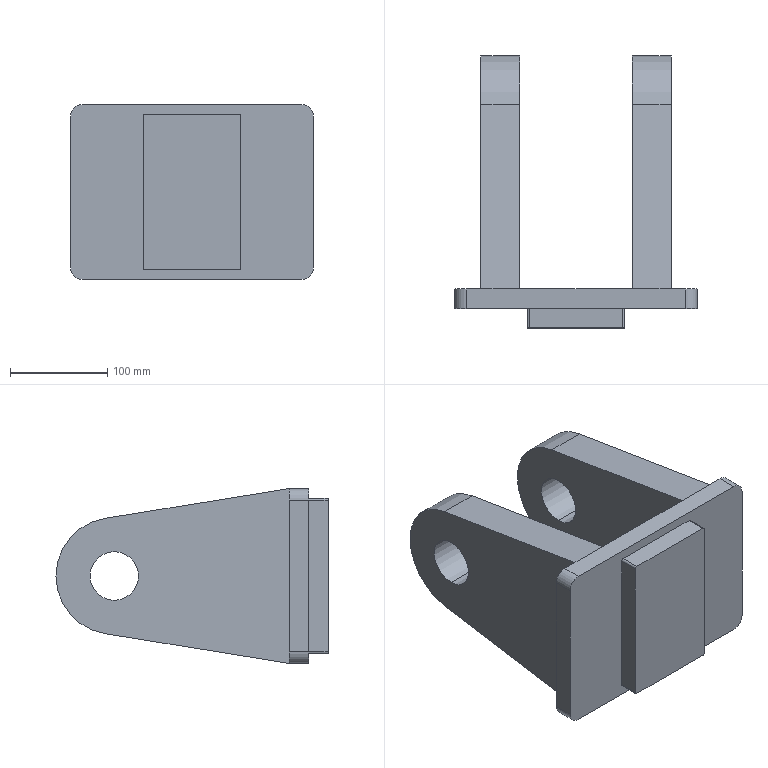Part | SolidWorks | features ICE 2, Extrusion 1, MirrorPattern 1 | 1 solid | 35 faces | box 250 x 280 x 180 mm | volume 3684479 mm3 | plane 21 | cylinder 14 | commonest cylinder face diameters 4 x4 24 x4 50 x4 120 x2
STEP:
#1=CARTESIAN_POINT('',(-98.,200.,25.));
#2=VERTEX_POINT('',#1);
#3=CARTESIAN_POINT('',(-98.,200.,-25.));
#4=VERTEX_POINT('',#3);
#5=CARTESIAN_POINT('',(-98.,200.,0.));
#6=DIRECTION('',(1.,0.,0.));
#7=DIRECTION('',(0.,0.,-1.));
#8=AXIS2_PLACEMENT_3D('',#5,#6,#7);
#9=CIRCLE('',#8,25.);
#10=EDGE_CURVE('',#2,#4,#9,.T.);
#11=ORIENTED_EDGE('',*,*,#10,.F.);
#12=CARTESIAN_POINT('',(-58.,200.,25.));
#13=VERTEX_POINT('',#12);
#14=CARTESIAN_POINT('',(-98.,200.,25.));
#15=DIRECTION('',(1.,0.,0.));
#16=VECTOR('',#15,1000.);
#17=LINE('',#14,#16);
#18=EDGE_CURVE('',#2,#13,#17,.T.);
#19=ORIENTED_EDGE('',*,*,#18,.T.);
#20=CARTESIAN_POINT('',(-58.,200.,-25.));
#21=VERTEX_POINT('',#20);
#22=CARTESIAN_POINT('',(-58.,200.,0.));
#23=DIRECTION('',(1.,0.,0.));
#24=DIRECTION('',(0.,0.,-1.));
#25=AXIS2_PLACEMENT_3D('',#22,#23,#24);
#26=CIRCLE('',#25,25.);
#27=EDGE_CURVE('',#13,#21,#26,.T.);
#28=ORIENTED_EDGE('',*,*,#27,.T.);
#29=CARTESIAN_POINT('',(-98.,200.,-25.));
#30=DIRECTION('',(1.,0.,0.));
#31=VECTOR('',#30,1000.);
#32=LINE('',#29,#31);
#33=EDGE_CURVE('',#4,#21,#32,.T.);
#34=ORIENTED_EDGE('',*,*,#33,.F.);
#35=EDGE_LOOP('',(#11,#19,#28,#34));
#36=FACE_OUTER_BOUND('',#35,.T.);
#37=CARTESIAN_POINT('',(-98.,200.,0.));
#38=DIRECTION('',(1.,0.,0.));
#39=DIRECTION('',(0.,0.,-1.));
#40=AXIS2_PLACEMENT_3D('',#37,#38,#39);
#41=CYLINDRICAL_SURFACE('',#40,25.);
#42=ADVANCED_FACE('',(#36),#41,.F.);
#43=CARTESIAN_POINT('',(98.,200.,25.));
#44=VERTEX_POINT('',#43);
#45=CARTESIAN_POINT('',(98.,200.,-25.));
#46=VERTEX_POINT('',#45);
#47=CARTESIAN_POINT('',(98.,200.,0.));
#48=DIRECTION('',(1.,0.,0.));
#49=DIRECTION('',(0.,0.,-1.));
#50=AXIS2_PLACEMENT_3D('',#47,#48,#49);
#51=CIRCLE('',#50,25.);
#52=EDGE_CURVE('',#44,#46,#51,.T.);
#53=ORIENTED_EDGE('',*,*,#52,.T.);
#54=CARTESIAN_POINT('',(58.,200.,-25.));
#55=VERTEX_POINT('',#54);
#56=CARTESIAN_POINT('',(98.,200.,-25.));
#57=DIRECTION('',(-1.,0.,0.));
#58=VECTOR('',#57,1000.);
#59=LINE('',#56,#58);
#60=EDGE_CURVE('',#46,#55,#59,.T.);
#61=ORIENTED_EDGE('',*,*,#60,.T.);
#62=CARTESIAN_POINT('',(58.,200.,25.));
#63=VERTEX_POINT('',#62);
#64=CARTESIAN_POINT('',(58.,200.,0.));
#65=DIRECTION('',(1.,0.,0.));
#66=DIRECTION('',(0.,0.,-1.));
#67=AXIS2_PLACEMENT_3D('',#64,#65,#66);
#68=CIRCLE('',#67,25.);
#69=EDGE_CURVE('',#63,#55,#68,.T.);
#70=ORIENTED_EDGE('',*,*,#69,.F.);
#71=CARTESIAN_POINT('',(98.,200.,25.));
#72=DIRECTION('',(-1.,0.,0.));
#73=VECTOR('',#72,1000.);
#74=LINE('',#71,#73);
#75=EDGE_CURVE('',#44,#63,#74,.T.);
#76=ORIENTED_EDGE('',*,*,#75,.F.);
#77=EDGE_LOOP('',(#53,#61,#70,#76));
#78=FACE_OUTER_BOUND('',#77,.T.);
#79=CARTESIAN_POINT('',(98.,200.,0.));
#80=DIRECTION('',(-1.,0.,0.));
#81=DIRECTION('',(0.,0.,1.));
#82=AXIS2_PLACEMENT_3D('',#79,#80,#81);
#83=CYLINDRICAL_SURFACE('',#82,25.);
#84=ADVANCED_FACE('',(#78),#83,.F.);
#85=CARTESIAN_POINT('',(58.,20.,-90.));
#86=VERTEX_POINT('',#85);
#87=CARTESIAN_POINT('',(-58.,20.,-90.));
#88=VERTEX_POINT('',#87);
#89=CARTESIAN_POINT('',(113.,20.,-90.));
#90=DIRECTION('',(-1.,0.,0.));
#91=VECTOR('',#90,1000.);
#92=LINE('',#89,#91);
#93=EDGE_CURVE('',#86,#88,#92,.T.);
#94=ORIENTED_EDGE('',*,*,#93,.T.);
#95=CARTESIAN_POINT('',(-58.,20.,90.));
#96=VERTEX_POINT('',#95);
#97=CARTESIAN_POINT('',(-58.,20.,90.));
#98=DIRECTION('',(0.,0.,-1.));
#99=VECTOR('',#98,1000.);
#100=LINE('',#97,#99);
#101=EDGE_CURVE('',#96,#88,#100,.T.);
#102=ORIENTED_EDGE('',*,*,#101,.F.);
#103=CARTESIAN_POINT('',(58.,20.,90.));
#104=VERTEX_POINT('',#103);
#105=CARTESIAN_POINT('',(113.,20.,90.));
#106=DIRECTION('',(1.,0.,0.));
#107=VECTOR('',#106,1000.);
#108=LINE('',#105,#107);
#109=EDGE_CURVE('',#96,#104,#108,.T.);
#110=ORIENTED_EDGE('',*,*,#109,.T.);
#111=CARTESIAN_POINT('',(58.,20.,90.));
#112=DIRECTION('',(0.,0.,-1.));
#113=VECTOR('',#112,1000.);
#114=LINE('',#111,#113);
#115=EDGE_CURVE('',#104,#86,#114,.T.);
#116=ORIENTED_EDGE('',*,*,#115,.T.);
#117=EDGE_LOOP('',(#94,#102,#110,#116));
#118=FACE_OUTER_BOUND('',#117,.T.);
#119=CARTESIAN_POINT('',(-113.,20.,-78.));
#120=DIRECTION('',(0.,1.,0.));
#121=DIRECTION('',(0.,0.,1.));
#122=AXIS2_PLACEMENT_3D('',#119,#120,#121);
#123=PLANE('',#122);
#124=ADVANCED_FACE('',(#118),#123,.T.);
#125=CARTESIAN_POINT('',(-98.,20.,90.));
#126=VERTEX_POINT('',#125);
#127=CARTESIAN_POINT('',(-98.,20.,-90.));
#128=VERTEX_POINT('',#127);
#129=CARTESIAN_POINT('',(-98.,20.,90.));
#130=DIRECTION('',(0.,0.,-1.));
#131=VECTOR('',#130,1000.);
#132=LINE('',#129,#131);
#133=EDGE_CURVE('',#126,#128,#132,.T.);
#134=ORIENTED_EDGE('',*,*,#133,.T.);
#135=CARTESIAN_POINT('',(-113.,20.,-90.));
#136=VERTEX_POINT('',#135);
#137=CARTESIAN_POINT('',(113.,20.,-90.));
#138=DIRECTION('',(-1.,0.,0.));
#139=VECTOR('',#138,1000.);
#140=LINE('',#137,#139);
#141=EDGE_CURVE('',#128,#136,#140,.T.);
#142=ORIENTED_EDGE('',*,*,#141,.T.);
#143=CARTESIAN_POINT('',(-125.,20.,-78.));
#144=VERTEX_POINT('',#143);
#145=CARTESIAN_POINT('',(-113.,20.,-78.));
#146=DIRECTION('',(0.,1.,0.));
#147=DIRECTION('',(0.,0.,1.));
#148=AXIS2_PLACEMENT_3D('',#145,#146,#147);
#149=CIRCLE('',#148,12.);
#150=EDGE_CURVE('',#136,#144,#149,.T.);
#151=ORIENTED_EDGE('',*,*,#150,.T.);
#152=CARTESIAN_POINT('',(-125.,20.,78.));
#153=VERTEX_POINT('',#152);
#154=CARTESIAN_POINT('',(-125.,20.,-78.));
#155=DIRECTION('',(0.,0.,1.));
#156=VECTOR('',#155,1000.);
#157=LINE('',#154,#156);
#158=EDGE_CURVE('',#144,#153,#157,.T.);
#159=ORIENTED_EDGE('',*,*,#158,.T.);
#160=CARTESIAN_POINT('',(-113.,20.,90.));
#161=VERTEX_POINT('',#160);
#162=CARTESIAN_POINT('',(-113.,20.,78.));
#163=DIRECTION('',(0.,1.,0.));
#164=DIRECTION('',(0.,0.,-1.));
#165=AXIS2_PLACEMENT_3D('',#162,#163,#164);
#166=CIRCLE('',#165,12.);
#167=EDGE_CURVE('',#153,#161,#166,.T.);
#168=ORIENTED_EDGE('',*,*,#167,.T.);
#169=CARTESIAN_POINT('',(113.,20.,90.));
#170=DIRECTION('',(1.,0.,0.));
#171=VECTOR('',#170,1000.);
#172=LINE('',#169,#171);
#173=EDGE_CURVE('',#161,#126,#172,.T.);
#174=ORIENTED_EDGE('',*,*,#173,.T.);
#175=EDGE_LOOP('',(#134,#142,#151,#159,#168,#174));
#176=FACE_OUTER_BOUND('',#175,.T.);
#177=CARTESIAN_POINT('',(-113.,20.,-78.));
#178=DIRECTION('',(0.,1.,0.));
#179=DIRECTION('',(0.,0.,1.));
#180=AXIS2_PLACEMENT_3D('',#177,#178,#179);
#181=PLANE('',#180);
#182=ADVANCED_FACE('',(#176),#181,.T.);
#183=CARTESIAN_POINT('',(-113.,0.,-90.));
#184=VERTEX_POINT('',#183);
#185=CARTESIAN_POINT('',(-125.,0.,-78.));
#186=VERTEX_POINT('',#185);
#187=CARTESIAN_POINT('',(-113.,0.,-78.));
#188=DIRECTION('',(0.,1.,0.));
#189=DIRECTION('',(0.,0.,1.));
#190=AXIS2_PLACEMENT_3D('',#187,#188,#189);
#191=CIRCLE('',#190,12.);
#192=EDGE_CURVE('',#184,#186,#191,.T.);
#193=ORIENTED_EDGE('',*,*,#192,.F.);
#194=CARTESIAN_POINT('',(113.,0.,-90.));
#195=VERTEX_POINT('',#194);
#196=CARTESIAN_POINT('',(113.,0.,-90.));
#197=DIRECTION('',(-1.,0.,0.));
#198=VECTOR('',#197,1000.);
#199=LINE('',#196,#198);
#200=EDGE_CURVE('',#195,#184,#199,.T.);
#201=ORIENTED_EDGE('',*,*,#200,.F.);
#202=CARTESIAN_POINT('',(125.,0.,-78.));
#203=VERTEX_POINT('',#202);
#204=CARTESIAN_POINT('',(113.,0.,-78.));
#205=DIRECTION('',(0.,1.,0.));
#206=DIRECTION('',(0.,0.,-1.));
#207=AXIS2_PLACEMENT_3D('',#204,#205,#206);
#208=CIRCLE('',#207,12.);
#209=EDGE_CURVE('',#203,#195,#208,.T.);
#210=ORIENTED_EDGE('',*,*,#209,.F.);
#211=CARTESIAN_POINT('',(125.,0.,78.));
#212=VERTEX_POINT('',#211);
#213=CARTESIAN_POINT('',(125.,0.,-78.));
#214=DIRECTION('',(0.,0.,-1.));
#215=VECTOR('',#214,1000.);
#216=LINE('',#213,#215);
#217=EDGE_CURVE('',#212,#203,#216,.T.);
#218=ORIENTED_EDGE('',*,*,#217,.F.);
#219=CARTESIAN_POINT('',(113.,0.,90.));
#220=VERTEX_POINT('',#219);
#221=CARTESIAN_POINT('',(113.,0.,78.));
#222=DIRECTION('',(0.,1.,0.));
#223=DIRECTION('',(0.,0.,1.));
#224=AXIS2_PLACEMENT_3D('',#221,#222,#223);
#225=CIRCLE('',#224,12.);
#226=EDGE_CURVE('',#220,#212,#225,.T.);
#227=ORIENTED_EDGE('',*,*,#226,.F.);
#228=CARTESIAN_POINT('',(-113.,0.,90.));
#229=VERTEX_POINT('',#228);
#230=CARTESIAN_POINT('',(113.,0.,90.));
#231=DIRECTION('',(1.,0.,0.));
#232=VECTOR('',#231,1000.);
#233=LINE('',#230,#232);
#234=EDGE_CURVE('',#229,#220,#233,.T.);
#235=ORIENTED_EDGE('',*,*,#234,.F.);
#236=CARTESIAN_POINT('',(-125.,0.,78.));
#237=VERTEX_POINT('',#236);
#238=CARTESIAN_POINT('',(-113.,0.,78.));
#239=DIRECTION('',(0.,1.,0.));
#240=DIRECTION('',(0.,0.,-1.));
#241=AXIS2_PLACEMENT_3D('',#238,#239,#240);
#242=CIRCLE('',#241,12.);
#243=EDGE_CURVE('',#237,#229,#242,.T.);
#244=ORIENTED_EDGE('',*,*,#243,.F.);
#245=CARTESIAN_POINT('',(-125.,0.,-78.));
#246=DIRECTION('',(0.,0.,1.));
#247=VECTOR('',#246,1000.);
#248=LINE('',#245,#247);
#249=EDGE_CURVE('',#186,#237,#248,.T.);
#250=ORIENTED_EDGE('',*,*,#249,.F.);
#251=EDGE_LOOP('',(#193,#201,#210,#218,#227,#235,#244,#250));
#252=FACE_OUTER_BOUND('',#251,.T.);
#253=CARTESIAN_POINT('',(-48.,0.,80.));
#254=VERTEX_POINT('',#253);
#255=CARTESIAN_POINT('',(-50.,0.,78.));
#256=VERTEX_POINT('',#255);
#257=CARTESIAN_POINT('',(-48.,0.,78.));
#258=DIRECTION('',(0.,-1.,0.));
#259=DIRECTION('',(0.,0.,-1.));
#260=AXIS2_PLACEMENT_3D('',#257,#258,#259);
#261=CIRCLE('',#260,2.);
#262=EDGE_CURVE('',#254,#256,#261,.T.);
#263=ORIENTED_EDGE('',*,*,#262,.F.);
#264=CARTESIAN_POINT('',(48.,0.,80.));
#265=VERTEX_POINT('',#264);
#266=CARTESIAN_POINT('',(48.,0.,80.));
#267=DIRECTION('',(-1.,0.,0.));
#268=VECTOR('',#267,1000.);
#269=LINE('',#266,#268);
#270=EDGE_CURVE('',#265,#254,#269,.T.);
#271=ORIENTED_EDGE('',*,*,#270,.F.);
#272=CARTESIAN_POINT('',(50.,0.,78.));
#273=VERTEX_POINT('',#272);
#274=CARTESIAN_POINT('',(48.,0.,78.));
#275=DIRECTION('',(0.,-1.,0.));
#276=DIRECTION('',(0.,0.,1.));
#277=AXIS2_PLACEMENT_3D('',#274,#275,#276);
#278=CIRCLE('',#277,2.);
#279=EDGE_CURVE('',#273,#265,#278,.T.);
#280=ORIENTED_EDGE('',*,*,#279,.F.);
#281=CARTESIAN_POINT('',(50.,0.,-78.));
#282=VERTEX_POINT('',#281);
#283=CARTESIAN_POINT('',(50.,0.,78.));
#284=DIRECTION('',(0.,0.,1.));
#285=VECTOR('',#284,1000.);
#286=LINE('',#283,#285);
#287=EDGE_CURVE('',#282,#273,#286,.T.);
#288=ORIENTED_EDGE('',*,*,#287,.F.);
#289=CARTESIAN_POINT('',(48.,0.,-80.));
#290=VERTEX_POINT('',#289);
#291=CARTESIAN_POINT('',(48.,0.,-78.));
#292=DIRECTION('',(0.,-1.,0.));
#293=DIRECTION('',(0.,0.,-1.));
#294=AXIS2_PLACEMENT_3D('',#291,#292,#293);
#295=CIRCLE('',#294,2.);
#296=EDGE_CURVE('',#290,#282,#295,.T.);
#297=ORIENTED_EDGE('',*,*,#296,.F.);
#298=CARTESIAN_POINT('',(-48.,0.,-80.));
#299=VERTEX_POINT('',#298);
#300=CARTESIAN_POINT('',(48.,0.,-80.));
#301=DIRECTION('',(1.,0.,0.));
#302=VECTOR('',#301,1000.);
#303=LINE('',#300,#302);
#304=EDGE_CURVE('',#299,#290,#303,.T.);
#305=ORIENTED_EDGE('',*,*,#304,.F.);
#306=CARTESIAN_POINT('',(-50.,0.,-78.));
#307=VERTEX_POINT('',#306);
#308=CARTESIAN_POINT('',(-48.,0.,-78.));
#309=DIRECTION('',(0.,-1.,0.));
#310=DIRECTION('',(0.,0.,1.));
#311=AXIS2_PLACEMENT_3D('',#308,#309,#310);
#312=CIRCLE('',#311,2.);
#313=EDGE_CURVE('',#307,#299,#312,.T.);
#314=ORIENTED_EDGE('',*,*,#313,.F.);
#315=CARTESIAN_POINT('',(-50.,0.,78.));
#316=DIRECTION('',(0.,0.,-1.));
#317=VECTOR('',#316,1000.);
#318=LINE('',#315,#317);
#319=EDGE_CURVE('',#256,#307,#318,.T.);
#320=ORIENTED_EDGE('',*,*,#319,.F.);
#321=EDGE_LOOP('',(#263,#271,#280,#288,#297,#305,#314,#320));
#322=FACE_BOUND('',#321,.T.);
#323=CARTESIAN_POINT('',(-113.,0.,-78.));
#324=DIRECTION('',(0.,1.,0.));
#325=DIRECTION('',(0.,0.,1.));
#326=AXIS2_PLACEMENT_3D('',#323,#324,#325);
#327=PLANE('',#326);
#328=ADVANCED_FACE('',(#252,#322),#327,.F.);
#329=ORIENTED_EDGE('',*,*,#192,.T.);
#330=CARTESIAN_POINT('',(-125.,20.,-78.));
#331=DIRECTION('',(0.,-1.,0.));
#332=VECTOR('',#331,1000.);
#333=LINE('',#330,#332);
#334=EDGE_CURVE('',#144,#186,#333,.T.);
#335=ORIENTED_EDGE('',*,*,#334,.F.);
#336=ORIENTED_EDGE('',*,*,#150,.F.);
#337=CARTESIAN_POINT('',(-113.,20.,-90.));
#338=DIRECTION('',(0.,-1.,0.));
#339=VECTOR('',#338,1000.);
#340=LINE('',#337,#339);
#341=EDGE_CURVE('',#136,#184,#340,.T.);
#342=ORIENTED_EDGE('',*,*,#341,.T.);
#343=EDGE_LOOP('',(#329,#335,#336,#342));
#344=FACE_OUTER_BOUND('',#343,.T.);
#345=CARTESIAN_POINT('',(-113.,20.,-78.));
#346=DIRECTION('',(0.,-1.,0.));
#347=DIRECTION('',(0.,0.,-1.));
#348=AXIS2_PLACEMENT_3D('',#345,#346,#347);
#349=CYLINDRICAL_SURFACE('',#348,12.);
#350=ADVANCED_FACE('',(#344),#349,.T.);
#351=ORIENTED_EDGE('',*,*,#249,.T.);
#352=CARTESIAN_POINT('',(-125.,20.,78.));
#353=DIRECTION('',(0.,-1.,0.));
#354=VECTOR('',#353,1000.);
#355=LINE('',#352,#354);
#356=EDGE_CURVE('',#153,#237,#355,.T.);
#357=ORIENTED_EDGE('',*,*,#356,.F.);
#358=ORIENTED_EDGE('',*,*,#158,.F.);
#359=ORIENTED_EDGE('',*,*,#334,.T.);
#360=EDGE_LOOP('',(#351,#357,#358,#359));
#361=FACE_OUTER_BOUND('',#360,.T.);
#362=CARTESIAN_POINT('',(-125.,20.,-78.));
#363=DIRECTION('',(1.,0.,0.));
#364=DIRECTION('',(0.,0.,-1.));
#365=AXIS2_PLACEMENT_3D('',#362,#363,#364);
#366=PLANE('',#365);
#367=ADVANCED_FACE('',(#361),#366,.F.);
#368=ORIENTED_EDGE('',*,*,#243,.T.);
#369=CARTESIAN_POINT('',(-113.,20.,90.));
#370=DIRECTION('',(0.,-1.,0.));
#371=VECTOR('',#370,1000.);
#372=LINE('',#369,#371);
#373=EDGE_CURVE('',#161,#229,#372,.T.);
#374=ORIENTED_EDGE('',*,*,#373,.F.);
#375=ORIENTED_EDGE('',*,*,#167,.F.);
#376=ORIENTED_EDGE('',*,*,#356,.T.);
#377=EDGE_LOOP('',(#368,#374,#375,#376));
#378=FACE_OUTER_BOUND('',#377,.T.);
#379=CARTESIAN_POINT('',(-113.,20.,78.));
#380=DIRECTION('',(0.,-1.,0.));
#381=DIRECTION('',(0.,0.,-1.));
#382=AXIS2_PLACEMENT_3D('',#379,#380,#381);
#383=CYLINDRICAL_SURFACE('',#382,12.);
#384=ADVANCED_FACE('',(#378),#383,.T.);
#385=ORIENTED_EDGE('',*,*,#234,.T.);
#386=CARTESIAN_POINT('',(113.,20.,90.));
#387=VERTEX_POINT('',#386);
#388=CARTESIAN_POINT('',(113.,20.,90.));
#389=DIRECTION('',(0.,-1.,0.));
#390=VECTOR('',#389,1000.);
#391=LINE('',#388,#390);
#392=EDGE_CURVE('',#387,#220,#391,.T.);
#393=ORIENTED_EDGE('',*,*,#392,.F.);
#394=CARTESIAN_POINT('',(98.,20.,90.));
#395=VERTEX_POINT('',#394);
#396=CARTESIAN_POINT('',(113.,20.,90.));
#397=DIRECTION('',(1.,0.,0.));
#398=VECTOR('',#397,1000.);
#399=LINE('',#396,#398);
#400=EDGE_CURVE('',#395,#387,#399,.T.);
#401=ORIENTED_EDGE('',*,*,#400,.F.);
#402=CARTESIAN_POINT('',(98.,20.,90.));
#403=DIRECTION('',(-1.,0.,0.));
#404=VECTOR('',#403,1000.);
#405=LINE('',#402,#404);
#406=EDGE_CURVE('',#395,#104,#405,.T.);
#407=ORIENTED_EDGE('',*,*,#406,.T.);
#408=ORIENTED_EDGE('',*,*,#109,.F.);
#409=CARTESIAN_POINT('',(-98.,20.,90.));
#410=DIRECTION('',(1.,0.,0.));
#411=VECTOR('',#410,1000.);
#412=LINE('',#409,#411);
#413=EDGE_CURVE('',#126,#96,#412,.T.);
#414=ORIENTED_EDGE('',*,*,#413,.F.);
#415=ORIENTED_EDGE('',*,*,#173,.F.);
#416=ORIENTED_EDGE('',*,*,#373,.T.);
#417=EDGE_LOOP('',(#385,#393,#401,#407,#408,#414,#415,#416));
#418=FACE_OUTER_BOUND('',#417,.T.);
#419=CARTESIAN_POINT('',(113.,20.,90.));
#420=DIRECTION('',(0.,0.,-1.));
#421=DIRECTION('',(-1.,0.,0.));
#422=AXIS2_PLACEMENT_3D('',#419,#420,#421);
#423=PLANE('',#422);
#424=ADVANCED_FACE('',(#418),#423,.F.);
#425=ORIENTED_EDGE('',*,*,#226,.T.);
#426=CARTESIAN_POINT('',(125.,20.,78.));
#427=VERTEX_POINT('',#426);
#428=CARTESIAN_POINT('',(125.,20.,78.));
#429=DIRECTION('',(0.,-1.,0.));
#430=VECTOR('',#429,1000.);
#431=LINE('',#428,#430);
#432=EDGE_CURVE('',#427,#212,#431,.T.);
#433=ORIENTED_EDGE('',*,*,#432,.F.);
#434=CARTESIAN_POINT('',(113.,20.,78.));
#435=DIRECTION('',(0.,1.,0.));
#436=DIRECTION('',(0.,0.,1.));
#437=AXIS2_PLACEMENT_3D('',#434,#435,#436);
#438=CIRCLE('',#437,12.);
#439=EDGE_CURVE('',#387,#427,#438,.T.);
#440=ORIENTED_EDGE('',*,*,#439,.F.);
#441=ORIENTED_EDGE('',*,*,#392,.T.);
#442=EDGE_LOOP('',(#425,#433,#440,#441));
#443=FACE_OUTER_BOUND('',#442,.T.);
#444=CARTESIAN_POINT('',(113.,20.,78.));
#445=DIRECTION('',(0.,-1.,0.));
#446=DIRECTION('',(0.,0.,-1.));
#447=AXIS2_PLACEMENT_3D('',#444,#445,#446);
#448=CYLINDRICAL_SURFACE('',#447,12.);
#449=ADVANCED_FACE('',(#443),#448,.T.);
#450=ORIENTED_EDGE('',*,*,#217,.T.);
#451=CARTESIAN_POINT('',(125.,20.,-78.));
#452=VERTEX_POINT('',#451);
#453=CARTESIAN_POINT('',(125.,20.,-78.));
#454=DIRECTION('',(0.,-1.,0.));
#455=VECTOR('',#454,1000.);
#456=LINE('',#453,#455);
#457=EDGE_CURVE('',#452,#203,#456,.T.);
#458=ORIENTED_EDGE('',*,*,#457,.F.);
#459=CARTESIAN_POINT('',(125.,20.,-78.));
#460=DIRECTION('',(0.,0.,-1.));
#461=VECTOR('',#460,1000.);
#462=LINE('',#459,#461);
#463=EDGE_CURVE('',#427,#452,#462,.T.);
#464=ORIENTED_EDGE('',*,*,#463,.F.);
#465=ORIENTED_EDGE('',*,*,#432,.T.);
#466=EDGE_LOOP('',(#450,#458,#464,#465));
#467=FACE_OUTER_BOUND('',#466,.T.);
#468=CARTESIAN_POINT('',(125.,20.,-78.));
#469=DIRECTION('',(-1.,0.,0.));
#470=DIRECTION('',(0.,0.,1.));
#471=AXIS2_PLACEMENT_3D('',#468,#469,#470);
#472=PLANE('',#471);
#473=ADVANCED_FACE('',(#467),#472,.F.);
#474=ORIENTED_EDGE('',*,*,#209,.T.);
#475=CARTESIAN_POINT('',(113.,20.,-90.));
#476=VERTEX_POINT('',#475);
#477=CARTESIAN_POINT('',(113.,20.,-90.));
#478=DIRECTION('',(0.,-1.,0.));
#479=VECTOR('',#478,1000.);
#480=LINE('',#477,#479);
#481=EDGE_CURVE('',#476,#195,#480,.T.);
#482=ORIENTED_EDGE('',*,*,#481,.F.);
#483=CARTESIAN_POINT('',(113.,20.,-78.));
#484=DIRECTION('',(0.,1.,0.));
#485=DIRECTION('',(0.,0.,-1.));
#486=AXIS2_PLACEMENT_3D('',#483,#484,#485);
#487=CIRCLE('',#486,12.);
#488=EDGE_CURVE('',#452,#476,#487,.T.);
#489=ORIENTED_EDGE('',*,*,#488,.F.);
#490=ORIENTED_EDGE('',*,*,#457,.T.);
#491=EDGE_LOOP('',(#474,#482,#489,#490));
#492=FACE_OUTER_BOUND('',#491,.T.);
#493=CARTESIAN_POINT('',(113.,20.,-78.));
#494=DIRECTION('',(0.,-1.,0.));
#495=DIRECTION('',(0.,0.,-1.));
#496=AXIS2_PLACEMENT_3D('',#493,#494,#495);
#497=CYLINDRICAL_SURFACE('',#496,12.);
#498=ADVANCED_FACE('',(#492),#497,.T.);
#499=ORIENTED_EDGE('',*,*,#200,.T.);
#500=ORIENTED_EDGE('',*,*,#341,.F.);
#501=ORIENTED_EDGE('',*,*,#141,.F.);
#502=CARTESIAN_POINT('',(-98.,20.,-90.));
#503=DIRECTION('',(1.,0.,0.));
#504=VECTOR('',#503,1000.);
#505=LINE('',#502,#504);
#506=EDGE_CURVE('',#128,#88,#505,.T.);
#507=ORIENTED_EDGE('',*,*,#506,.T.);
#508=ORIENTED_EDGE('',*,*,#93,.F.);
#509=CARTESIAN_POINT('',(98.,20.,-90.));
#510=VERTEX_POINT('',#509);
#511=CARTESIAN_POINT('',(98.,20.,-90.));
#512=DIRECTION('',(-1.,0.,0.));
#513=VECTOR('',#512,1000.);
#514=LINE('',#511,#513);
#515=EDGE_CURVE('',#510,#86,#514,.T.);
#516=ORIENTED_EDGE('',*,*,#515,.F.);
#517=CARTESIAN_POINT('',(113.,20.,-90.));
#518=DIRECTION('',(-1.,0.,0.));
#519=VECTOR('',#518,1000.);
#520=LINE('',#517,#519);
#521=EDGE_CURVE('',#476,#510,#520,.T.);
#522=ORIENTED_EDGE('',*,*,#521,.F.);
#523=ORIENTED_EDGE('',*,*,#481,.T.);
#524=EDGE_LOOP('',(#499,#500,#501,#507,#508,#516,#522,#523));
#525=FACE_OUTER_BOUND('',#524,.T.);
#526=CARTESIAN_POINT('',(113.,20.,-90.));
#527=DIRECTION('',(0.,0.,1.));
#528=DIRECTION('',(1.,0.,0.));
#529=AXIS2_PLACEMENT_3D('',#526,#527,#528);
#530=PLANE('',#529);
#531=ADVANCED_FACE('',(#525),#530,.F.);
#532=CARTESIAN_POINT('',(98.,20.,90.));
#533=DIRECTION('',(0.,0.,-1.));
#534=VECTOR('',#533,1000.);
#535=LINE('',#532,#534);
#536=EDGE_CURVE('',#395,#510,#535,.T.);
#537=ORIENTED_EDGE('',*,*,#536,.F.);
#538=ORIENTED_EDGE('',*,*,#400,.T.);
#539=ORIENTED_EDGE('',*,*,#439,.T.);
#540=ORIENTED_EDGE('',*,*,#463,.T.);
#541=ORIENTED_EDGE('',*,*,#488,.T.);
#542=ORIENTED_EDGE('',*,*,#521,.T.);
#543=EDGE_LOOP('',(#537,#538,#539,#540,#541,#542));
#544=FACE_OUTER_BOUND('',#543,.T.);
#545=CARTESIAN_POINT('',(-113.,20.,-78.));
#546=DIRECTION('',(0.,1.,0.));
#547=DIRECTION('',(0.,0.,1.));
#548=AXIS2_PLACEMENT_3D('',#545,#546,#547);
#549=PLANE('',#548);
#550=ADVANCED_FACE('',(#544),#549,.T.);
#551=ORIENTED_EDGE('',*,*,#262,.T.);
#552=CARTESIAN_POINT('',(-50.,-20.,78.));
#553=VERTEX_POINT('',#552);
#554=CARTESIAN_POINT('',(-50.,-20.,78.));
#555=DIRECTION('',(0.,1.,0.));
#556=VECTOR('',#555,1000.);
#557=LINE('',#554,#556);
#558=EDGE_CURVE('',#553,#256,#557,.T.);
#559=ORIENTED_EDGE('',*,*,#558,.F.);
#560=CARTESIAN_POINT('',(-48.,-20.,80.));
#561=VERTEX_POINT('',#560);
#562=CARTESIAN_POINT('',(-48.,-20.,78.));
#563=DIRECTION('',(0.,-1.,0.));
#564=DIRECTION('',(0.,0.,-1.));
#565=AXIS2_PLACEMENT_3D('',#562,#563,#564);
#566=CIRCLE('',#565,2.);
#567=EDGE_CURVE('',#561,#553,#566,.T.);
#568=ORIENTED_EDGE('',*,*,#567,.F.);
#569=CARTESIAN_POINT('',(-48.,-20.,80.));
#570=DIRECTION('',(0.,1.,0.));
#571=VECTOR('',#570,1000.);
#572=LINE('',#569,#571);
#573=EDGE_CURVE('',#561,#254,#572,.T.);
#574=ORIENTED_EDGE('',*,*,#573,.T.);
#575=EDGE_LOOP('',(#551,#559,#568,#574));
#576=FACE_OUTER_BOUND('',#575,.T.);
#577=CARTESIAN_POINT('',(-48.,-20.,78.));
#578=DIRECTION('',(0.,1.,0.));
#579=DIRECTION('',(0.,0.,1.));
#580=AXIS2_PLACEMENT_3D('',#577,#578,#579);
#581=CYLINDRICAL_SURFACE('',#580,2.);
#582=ADVANCED_FACE('',(#576),#581,.T.);
#583=ORIENTED_EDGE('',*,*,#319,.T.);
#584=CARTESIAN_POINT('',(-50.,-20.,-78.));
#585=VERTEX_POINT('',#584);
#586=CARTESIAN_POINT('',(-50.,-20.,-78.));
#587=DIRECTION('',(0.,1.,0.));
#588=VECTOR('',#587,1000.);
#589=LINE('',#586,#588);
#590=EDGE_CURVE('',#585,#307,#589,.T.);
#591=ORIENTED_EDGE('',*,*,#590,.F.);
#592=CARTESIAN_POINT('',(-50.,-20.,78.));
#593=DIRECTION('',(0.,0.,-1.));
#594=VECTOR('',#593,1000.);
#595=LINE('',#592,#594);
#596=EDGE_CURVE('',#553,#585,#595,.T.);
#597=ORIENTED_EDGE('',*,*,#596,.F.);
#598=ORIENTED_EDGE('',*,*,#558,.T.);
#599=EDGE_LOOP('',(#583,#591,#597,#598));
#600=FACE_OUTER_BOUND('',#599,.T.);
#601=CARTESIAN_POINT('',(-50.,-20.,78.));
#602=DIRECTION('',(1.,0.,0.));
#603=DIRECTION('',(0.,0.,-1.));
#604=AXIS2_PLACEMENT_3D('',#601,#602,#603);
#605=PLANE('',#604);
#606=ADVANCED_FACE('',(#600),#605,.F.);
#607=ORIENTED_EDGE('',*,*,#313,.T.);
#608=CARTESIAN_POINT('',(-48.,-20.,-80.));
#609=VERTEX_POINT('',#608);
#610=CARTESIAN_POINT('',(-48.,-20.,-80.));
#611=DIRECTION('',(0.,1.,0.));
#612=VECTOR('',#611,1000.);
#613=LINE('',#610,#612);
#614=EDGE_CURVE('',#609,#299,#613,.T.);
#615=ORIENTED_EDGE('',*,*,#614,.F.);
#616=CARTESIAN_POINT('',(-48.,-20.,-78.));
#617=DIRECTION('',(0.,-1.,0.));
#618=DIRECTION('',(0.,0.,1.));
#619=AXIS2_PLACEMENT_3D('',#616,#617,#618);
#620=CIRCLE('',#619,2.);
#621=EDGE_CURVE('',#585,#609,#620,.T.);
#622=ORIENTED_EDGE('',*,*,#621,.F.);
#623=ORIENTED_EDGE('',*,*,#590,.T.);
#624=EDGE_LOOP('',(#607,#615,#622,#623));
#625=FACE_OUTER_BOUND('',#624,.T.);
#626=CARTESIAN_POINT('',(-48.,-20.,-78.));
#627=DIRECTION('',(0.,1.,0.));
#628=DIRECTION('',(0.,0.,1.));
#629=AXIS2_PLACEMENT_3D('',#626,#627,#628);
#630=CYLINDRICAL_SURFACE('',#629,2.);
#631=ADVANCED_FACE('',(#625),#630,.T.);
#632=ORIENTED_EDGE('',*,*,#304,.T.);
#633=CARTESIAN_POINT('',(48.,-20.,-80.));
#634=VERTEX_POINT('',#633);
#635=CARTESIAN_POINT('',(48.,-20.,-80.));
#636=DIRECTION('',(0.,1.,0.));
#637=VECTOR('',#636,1000.);
#638=LINE('',#635,#637);
#639=EDGE_CURVE('',#634,#290,#638,.T.);
#640=ORIENTED_EDGE('',*,*,#639,.F.);
#641=CARTESIAN_POINT('',(48.,-20.,-80.));
#642=DIRECTION('',(1.,0.,0.));
#643=VECTOR('',#642,1000.);
#644=LINE('',#641,#643);
#645=EDGE_CURVE('',#609,#634,#644,.T.);
#646=ORIENTED_EDGE('',*,*,#645,.F.);
#647=ORIENTED_EDGE('',*,*,#614,.T.);
#648=EDGE_LOOP('',(#632,#640,#646,#647));
#649=FACE_OUTER_BOUND('',#648,.T.);
#650=CARTESIAN_POINT('',(48.,-20.,-80.));
#651=DIRECTION('',(0.,0.,1.));
#652=DIRECTION('',(1.,0.,0.));
#653=AXIS2_PLACEMENT_3D('',#650,#651,#652);
#654=PLANE('',#653);
#655=ADVANCED_FACE('',(#649),#654,.F.);
#656=ORIENTED_EDGE('',*,*,#296,.T.);
#657=CARTESIAN_POINT('',(50.,-20.,-78.));
#658=VERTEX_POINT('',#657);
#659=CARTESIAN_POINT('',(50.,-20.,-78.));
#660=DIRECTION('',(0.,1.,0.));
#661=VECTOR('',#660,1000.);
#662=LINE('',#659,#661);
#663=EDGE_CURVE('',#658,#282,#662,.T.);
#664=ORIENTED_EDGE('',*,*,#663,.F.);
#665=CARTESIAN_POINT('',(48.,-20.,-78.));
#666=DIRECTION('',(0.,-1.,0.));
#667=DIRECTION('',(0.,0.,-1.));
#668=AXIS2_PLACEMENT_3D('',#665,#666,#667);
#669=CIRCLE('',#668,2.);
#670=EDGE_CURVE('',#634,#658,#669,.T.);
#671=ORIENTED_EDGE('',*,*,#670,.F.);
#672=ORIENTED_EDGE('',*,*,#639,.T.);
#673=EDGE_LOOP('',(#656,#664,#671,#672));
#674=FACE_OUTER_BOUND('',#673,.T.);
#675=CARTESIAN_POINT('',(48.,-20.,-78.));
#676=DIRECTION('',(0.,1.,0.));
#677=DIRECTION('',(0.,0.,1.));
#678=AXIS2_PLACEMENT_3D('',#675,#676,#677);
#679=CYLINDRICAL_SURFACE('',#678,2.);
#680=ADVANCED_FACE('',(#674),#679,.T.);
#681=ORIENTED_EDGE('',*,*,#287,.T.);
#682=CARTESIAN_POINT('',(50.,-20.,78.));
#683=VERTEX_POINT('',#682);
#684=CARTESIAN_POINT('',(50.,-20.,78.));
#685=DIRECTION('',(0.,1.,0.));
#686=VECTOR('',#685,1000.);
#687=LINE('',#684,#686);
#688=EDGE_CURVE('',#683,#273,#687,.T.);
#689=ORIENTED_EDGE('',*,*,#688,.F.);
#690=CARTESIAN_POINT('',(50.,-20.,78.));
#691=DIRECTION('',(0.,0.,1.));
#692=VECTOR('',#691,1000.);
#693=LINE('',#690,#692);
#694=EDGE_CURVE('',#658,#683,#693,.T.);
#695=ORIENTED_EDGE('',*,*,#694,.F.);
#696=ORIENTED_EDGE('',*,*,#663,.T.);
#697=EDGE_LOOP('',(#681,#689,#695,#696));
#698=FACE_OUTER_BOUND('',#697,.T.);
#699=CARTESIAN_POINT('',(50.,-20.,78.));
#700=DIRECTION('',(-1.,0.,0.));
#701=DIRECTION('',(0.,0.,1.));
#702=AXIS2_PLACEMENT_3D('',#699,#700,#701);
#703=PLANE('',#702);
#704=ADVANCED_FACE('',(#698),#703,.F.);
#705=ORIENTED_EDGE('',*,*,#279,.T.);
#706=CARTESIAN_POINT('',(48.,-20.,80.));
#707=VERTEX_POINT('',#706);
#708=CARTESIAN_POINT('',(48.,-20.,80.));
#709=DIRECTION('',(0.,1.,0.));
#710=VECTOR('',#709,1000.);
#711=LINE('',#708,#710);
#712=EDGE_CURVE('',#707,#265,#711,.T.);
#713=ORIENTED_EDGE('',*,*,#712,.F.);
#714=CARTESIAN_POINT('',(48.,-20.,78.));
#715=DIRECTION('',(0.,-1.,0.));
#716=DIRECTION('',(0.,0.,1.));
#717=AXIS2_PLACEMENT_3D('',#714,#715,#716);
#718=CIRCLE('',#717,2.);
#719=EDGE_CURVE('',#683,#707,#718,.T.);
#720=ORIENTED_EDGE('',*,*,#719,.F.);
#721=ORIENTED_EDGE('',*,*,#688,.T.);
#722=EDGE_LOOP('',(#705,#713,#720,#721));
#723=FACE_OUTER_BOUND('',#722,.T.);
#724=CARTESIAN_POINT('',(48.,-20.,78.));
#725=DIRECTION('',(0.,1.,0.));
#726=DIRECTION('',(0.,0.,1.));
#727=AXIS2_PLACEMENT_3D('',#724,#725,#726);
#728=CYLINDRICAL_SURFACE('',#727,2.);
#729=ADVANCED_FACE('',(#723),#728,.T.);
#730=ORIENTED_EDGE('',*,*,#270,.T.);
#731=ORIENTED_EDGE('',*,*,#573,.F.);
#732=CARTESIAN_POINT('',(48.,-20.,80.));
#733=DIRECTION('',(-1.,0.,0.));
#734=VECTOR('',#733,1000.);
#735=LINE('',#732,#734);
#736=EDGE_CURVE('',#707,#561,#735,.T.);
#737=ORIENTED_EDGE('',*,*,#736,.F.);
#738=ORIENTED_EDGE('',*,*,#712,.T.);
#739=EDGE_LOOP('',(#730,#731,#737,#738));
#740=FACE_OUTER_BOUND('',#739,.T.);
#741=CARTESIAN_POINT('',(48.,-20.,80.));
#742=DIRECTION('',(0.,0.,-1.));
#743=DIRECTION('',(-1.,0.,0.));
#744=AXIS2_PLACEMENT_3D('',#741,#742,#743);
#745=PLANE('',#744);
#746=ADVANCED_FACE('',(#740),#745,.F.);
#747=ORIENTED_EDGE('',*,*,#567,.T.);
#748=ORIENTED_EDGE('',*,*,#596,.T.);
#749=ORIENTED_EDGE('',*,*,#621,.T.);
#750=ORIENTED_EDGE('',*,*,#645,.T.);
#751=ORIENTED_EDGE('',*,*,#670,.T.);
#752=ORIENTED_EDGE('',*,*,#694,.T.);
#753=ORIENTED_EDGE('',*,*,#719,.T.);
#754=ORIENTED_EDGE('',*,*,#736,.T.);
#755=EDGE_LOOP('',(#747,#748,#749,#750,#751,#752,#753,#754));
#756=FACE_OUTER_BOUND('',#755,.T.);
#757=CARTESIAN_POINT('',(-48.,-20.,78.));
#758=DIRECTION('',(0.,-1.,0.));
#759=DIRECTION('',(0.,0.,-1.));
#760=AXIS2_PLACEMENT_3D('',#757,#758,#759);
#761=PLANE('',#760);
#762=ADVANCED_FACE('',(#756),#761,.T.);
#763=CARTESIAN_POINT('',(98.,209.612,-59.225));
#764=VERTEX_POINT('',#763);
#765=CARTESIAN_POINT('',(98.,209.612,-59.225));
#766=DIRECTION('',(0.,0.9871,0.1602));
#767=VECTOR('',#766,1000.);
#768=LINE('',#765,#767);
#769=EDGE_CURVE('',#510,#764,#768,.T.);
#770=ORIENTED_EDGE('',*,*,#769,.T.);
#771=CARTESIAN_POINT('',(98.,209.612,59.225));
#772=VERTEX_POINT('',#771);
#773=CARTESIAN_POINT('',(98.,200.,0.));
#774=DIRECTION('',(1.,0.,0.));
#775=DIRECTION('',(0.,0.,-1.));
#776=AXIS2_PLACEMENT_3D('',#773,#774,#775);
#777=CIRCLE('',#776,60.);
#778=EDGE_CURVE('',#764,#772,#777,.T.);
#779=ORIENTED_EDGE('',*,*,#778,.T.);
#780=CARTESIAN_POINT('',(98.,209.612,59.225));
#781=DIRECTION('',(0.,-0.9871,0.1602));
#782=VECTOR('',#781,1000.);
#783=LINE('',#780,#782);
#784=EDGE_CURVE('',#772,#395,#783,.T.);
#785=ORIENTED_EDGE('',*,*,#784,.T.);
#786=ORIENTED_EDGE('',*,*,#536,.T.);
#787=EDGE_LOOP('',(#770,#779,#785,#786));
#788=FACE_OUTER_BOUND('',#787,.T.);
#789=ORIENTED_EDGE('',*,*,#52,.F.);
#790=CARTESIAN_POINT('',(98.,200.,0.));
#791=DIRECTION('',(1.,0.,0.));
#792=DIRECTION('',(0.,0.,-1.));
#793=AXIS2_PLACEMENT_3D('',#790,#791,#792);
#794=CIRCLE('',#793,25.);
#795=EDGE_CURVE('',#46,#44,#794,.T.);
#796=ORIENTED_EDGE('',*,*,#795,.F.);
#797=EDGE_LOOP('',(#789,#796));
#798=FACE_BOUND('',#797,.T.);
#799=CARTESIAN_POINT('',(98.,200.,0.));
#800=DIRECTION('',(1.,0.,0.));
#801=DIRECTION('',(0.,0.,-1.));
#802=AXIS2_PLACEMENT_3D('',#799,#800,#801);
#803=PLANE('',#802);
#804=ADVANCED_FACE('',(#788,#798),#803,.T.);
#805=CARTESIAN_POINT('',(58.,209.612,-59.225));
#806=VERTEX_POINT('',#805);
#807=CARTESIAN_POINT('',(58.,209.612,-59.225));
#808=DIRECTION('',(0.,0.9871,0.1602));
#809=VECTOR('',#808,1000.);
#810=LINE('',#807,#809);
#811=EDGE_CURVE('',#86,#806,#810,.T.);
#812=ORIENTED_EDGE('',*,*,#811,.F.);
#813=ORIENTED_EDGE('',*,*,#115,.F.);
#814=CARTESIAN_POINT('',(58.,209.612,59.225));
#815=VERTEX_POINT('',#814);
#816=CARTESIAN_POINT('',(58.,209.612,59.225));
#817=DIRECTION('',(0.,-0.9871,0.1602));
#818=VECTOR('',#817,1000.);
#819=LINE('',#816,#818);
#820=EDGE_CURVE('',#815,#104,#819,.T.);
#821=ORIENTED_EDGE('',*,*,#820,.F.);
#822=CARTESIAN_POINT('',(58.,200.,0.));
#823=DIRECTION('',(1.,0.,0.));
#824=DIRECTION('',(0.,0.,-1.));
#825=AXIS2_PLACEMENT_3D('',#822,#823,#824);
#826=CIRCLE('',#825,60.);
#827=EDGE_CURVE('',#806,#815,#826,.T.);
#828=ORIENTED_EDGE('',*,*,#827,.F.);
#829=EDGE_LOOP('',(#812,#813,#821,#828));
#830=FACE_OUTER_BOUND('',#829,.T.);
#831=ORIENTED_EDGE('',*,*,#69,.T.);
#832=CARTESIAN_POINT('',(58.,200.,0.));
#833=DIRECTION('',(1.,0.,0.));
#834=DIRECTION('',(0.,0.,-1.));
#835=AXIS2_PLACEMENT_3D('',#832,#833,#834);
#836=CIRCLE('',#835,25.);
#837=EDGE_CURVE('',#55,#63,#836,.T.);
#838=ORIENTED_EDGE('',*,*,#837,.T.);
#839=EDGE_LOOP('',(#831,#838));
#840=FACE_BOUND('',#839,.T.);
#841=CARTESIAN_POINT('',(58.,200.,0.));
#842=DIRECTION('',(1.,0.,0.));
#843=DIRECTION('',(0.,0.,-1.));
#844=AXIS2_PLACEMENT_3D('',#841,#842,#843);
#845=PLANE('',#844);
#846=ADVANCED_FACE('',(#830,#840),#845,.F.);
#847=ORIENTED_EDGE('',*,*,#811,.T.);
#848=CARTESIAN_POINT('',(98.,209.612,-59.225));
#849=DIRECTION('',(-1.,0.,0.));
#850=VECTOR('',#849,1000.);
#851=LINE('',#848,#850);
#852=EDGE_CURVE('',#764,#806,#851,.T.);
#853=ORIENTED_EDGE('',*,*,#852,.F.);
#854=ORIENTED_EDGE('',*,*,#769,.F.);
#855=ORIENTED_EDGE('',*,*,#515,.T.);
#856=EDGE_LOOP('',(#847,#853,#854,#855));
#857=FACE_OUTER_BOUND('',#856,.T.);
#858=CARTESIAN_POINT('',(98.,209.612,-59.225));
#859=DIRECTION('',(0.,-0.1602,0.9871));
#860=DIRECTION('',(0.,-0.9871,-0.1602));
#861=AXIS2_PLACEMENT_3D('',#858,#859,#860);
#862=PLANE('',#861);
#863=ADVANCED_FACE('',(#857),#862,.F.);
#864=ORIENTED_EDGE('',*,*,#827,.T.);
#865=CARTESIAN_POINT('',(98.,209.612,59.225));
#866=DIRECTION('',(-1.,0.,0.));
#867=VECTOR('',#866,1000.);
#868=LINE('',#865,#867);
#869=EDGE_CURVE('',#772,#815,#868,.T.);
#870=ORIENTED_EDGE('',*,*,#869,.F.);
#871=ORIENTED_EDGE('',*,*,#778,.F.);
#872=ORIENTED_EDGE('',*,*,#852,.T.);
#873=EDGE_LOOP('',(#864,#870,#871,#872));
#874=FACE_OUTER_BOUND('',#873,.T.);
#875=CARTESIAN_POINT('',(98.,200.,0.));
#876=DIRECTION('',(-1.,0.,0.));
#877=DIRECTION('',(0.,0.,1.));
#878=AXIS2_PLACEMENT_3D('',#875,#876,#877);
#879=CYLINDRICAL_SURFACE('',#878,60.);
#880=ADVANCED_FACE('',(#874),#879,.T.);
#881=ORIENTED_EDGE('',*,*,#820,.T.);
#882=ORIENTED_EDGE('',*,*,#406,.F.);
#883=ORIENTED_EDGE('',*,*,#784,.F.);
#884=ORIENTED_EDGE('',*,*,#869,.T.);
#885=EDGE_LOOP('',(#881,#882,#883,#884));
#886=FACE_OUTER_BOUND('',#885,.T.);
#887=CARTESIAN_POINT('',(98.,209.612,59.225));
#888=DIRECTION('',(0.,-0.1602,-0.9871));
#889=DIRECTION('',(0.,0.9871,-0.1602));
#890=AXIS2_PLACEMENT_3D('',#887,#888,#889);
#891=PLANE('',#890);
#892=ADVANCED_FACE('',(#886),#891,.F.);
#893=ORIENTED_EDGE('',*,*,#60,.F.);
#894=ORIENTED_EDGE('',*,*,#795,.T.);
#895=ORIENTED_EDGE('',*,*,#75,.T.);
#896=ORIENTED_EDGE('',*,*,#837,.F.);
#897=EDGE_LOOP('',(#893,#894,#895,#896));
#898=FACE_OUTER_BOUND('',#897,.T.);
#899=CARTESIAN_POINT('',(98.,200.,0.));
#900=DIRECTION('',(-1.,0.,0.));
#901=DIRECTION('',(0.,0.,1.));
#902=AXIS2_PLACEMENT_3D('',#899,#900,#901);
#903=CYLINDRICAL_SURFACE('',#902,25.);
#904=ADVANCED_FACE('',(#898),#903,.F.);
#905=CARTESIAN_POINT('',(-58.,209.612,-59.225));
#906=VERTEX_POINT('',#905);
#907=CARTESIAN_POINT('',(-58.,209.612,-59.225));
#908=DIRECTION('',(0.,0.9871,0.1602));
#909=VECTOR('',#908,1000.);
#910=LINE('',#907,#909);
#911=EDGE_CURVE('',#88,#906,#910,.T.);
#912=ORIENTED_EDGE('',*,*,#911,.F.);
#913=ORIENTED_EDGE('',*,*,#506,.F.);
#914=CARTESIAN_POINT('',(-98.,209.612,-59.225));
#915=VERTEX_POINT('',#914);
#916=CARTESIAN_POINT('',(-98.,209.612,-59.225));
#917=DIRECTION('',(0.,0.9871,0.1602));
#918=VECTOR('',#917,1000.);
#919=LINE('',#916,#918);
#920=EDGE_CURVE('',#128,#915,#919,.T.);
#921=ORIENTED_EDGE('',*,*,#920,.T.);
#922=CARTESIAN_POINT('',(-98.,209.612,-59.225));
#923=DIRECTION('',(1.,0.,0.));
#924=VECTOR('',#923,1000.);
#925=LINE('',#922,#924);
#926=EDGE_CURVE('',#915,#906,#925,.T.);
#927=ORIENTED_EDGE('',*,*,#926,.T.);
#928=EDGE_LOOP('',(#912,#913,#921,#927));
#929=FACE_OUTER_BOUND('',#928,.T.);
#930=CARTESIAN_POINT('',(-98.,209.612,-59.225));
#931=DIRECTION('',(0.,0.1602,-0.9871));
#932=DIRECTION('',(0.,0.9871,0.1602));
#933=AXIS2_PLACEMENT_3D('',#930,#931,#932);
#934=PLANE('',#933);
#935=ADVANCED_FACE('',(#929),#934,.T.);
#936=CARTESIAN_POINT('',(-58.,209.612,59.225));
#937=VERTEX_POINT('',#936);
#938=CARTESIAN_POINT('',(-58.,209.612,59.225));
#939=DIRECTION('',(0.,-0.9871,0.1602));
#940=VECTOR('',#939,1000.);
#941=LINE('',#938,#940);
#942=EDGE_CURVE('',#937,#96,#941,.T.);
#943=ORIENTED_EDGE('',*,*,#942,.F.);
#944=CARTESIAN_POINT('',(-98.,209.612,59.225));
#945=VERTEX_POINT('',#944);
#946=CARTESIAN_POINT('',(-98.,209.612,59.225));
#947=DIRECTION('',(1.,0.,0.));
#948=VECTOR('',#947,1000.);
#949=LINE('',#946,#948);
#950=EDGE_CURVE('',#945,#937,#949,.T.);
#951=ORIENTED_EDGE('',*,*,#950,.F.);
#952=CARTESIAN_POINT('',(-98.,209.612,59.225));
#953=DIRECTION('',(0.,-0.9871,0.1602));
#954=VECTOR('',#953,1000.);
#955=LINE('',#952,#954);
#956=EDGE_CURVE('',#945,#126,#955,.T.);
#957=ORIENTED_EDGE('',*,*,#956,.T.);
#958=ORIENTED_EDGE('',*,*,#413,.T.);
#959=EDGE_LOOP('',(#943,#951,#957,#958));
#960=FACE_OUTER_BOUND('',#959,.T.);
#961=CARTESIAN_POINT('',(-98.,209.612,59.225));
#962=DIRECTION('',(0.,0.1602,0.9871));
#963=DIRECTION('',(0.,-0.9871,0.1602));
#964=AXIS2_PLACEMENT_3D('',#961,#962,#963);
#965=PLANE('',#964);
#966=ADVANCED_FACE('',(#960),#965,.T.);
#967=CARTESIAN_POINT('',(-58.,200.,0.));
#968=DIRECTION('',(1.,0.,0.));
#969=DIRECTION('',(0.,0.,-1.));
#970=AXIS2_PLACEMENT_3D('',#967,#968,#969);
#971=CIRCLE('',#970,60.);
#972=EDGE_CURVE('',#906,#937,#971,.T.);
#973=ORIENTED_EDGE('',*,*,#972,.F.);
#974=ORIENTED_EDGE('',*,*,#926,.F.);
#975=CARTESIAN_POINT('',(-98.,200.,0.));
#976=DIRECTION('',(1.,0.,0.));
#977=DIRECTION('',(0.,0.,-1.));
#978=AXIS2_PLACEMENT_3D('',#975,#976,#977);
#979=CIRCLE('',#978,60.);
#980=EDGE_CURVE('',#915,#945,#979,.T.);
#981=ORIENTED_EDGE('',*,*,#980,.T.);
#982=ORIENTED_EDGE('',*,*,#950,.T.);
#983=EDGE_LOOP('',(#973,#974,#981,#982));
#984=FACE_OUTER_BOUND('',#983,.T.);
#985=CARTESIAN_POINT('',(-98.,200.,0.));
#986=DIRECTION('',(1.,0.,0.));
#987=DIRECTION('',(0.,0.,-1.));
#988=AXIS2_PLACEMENT_3D('',#985,#986,#987);
#989=CYLINDRICAL_SURFACE('',#988,60.);
#990=ADVANCED_FACE('',(#984),#989,.T.);
#991=CARTESIAN_POINT('',(-98.,200.,0.));
#992=DIRECTION('',(1.,0.,0.));
#993=DIRECTION('',(0.,0.,-1.));
#994=AXIS2_PLACEMENT_3D('',#991,#992,#993);
#995=CIRCLE('',#994,25.);
#996=EDGE_CURVE('',#4,#2,#995,.T.);
#997=ORIENTED_EDGE('',*,*,#996,.T.);
#998=ORIENTED_EDGE('',*,*,#10,.T.);
#999=EDGE_LOOP('',(#997,#998));
#1000=FACE_BOUND('',#999,.T.);
#1001=ORIENTED_EDGE('',*,*,#920,.F.);
#1002=ORIENTED_EDGE('',*,*,#133,.F.);
#1003=ORIENTED_EDGE('',*,*,#956,.F.);
#1004=ORIENTED_EDGE('',*,*,#980,.F.);
#1005=EDGE_LOOP('',(#1001,#1002,#1003,#1004));
#1006=FACE_OUTER_BOUND('',#1005,.T.);
#1007=CARTESIAN_POINT('',(-98.,200.,0.));
#1008=DIRECTION('',(-1.,0.,0.));
#1009=DIRECTION('',(0.,0.,-1.));
#1010=AXIS2_PLACEMENT_3D('',#1007,#1008,#1009);
#1011=PLANE('',#1010);
#1012=ADVANCED_FACE('',(#1000,#1006),#1011,.T.);
#1013=CARTESIAN_POINT('',(-58.,200.,0.));
#1014=DIRECTION('',(1.,0.,0.));
#1015=DIRECTION('',(0.,0.,-1.));
#1016=AXIS2_PLACEMENT_3D('',#1013,#1014,#1015);
#1017=CIRCLE('',#1016,25.);
#1018=EDGE_CURVE('',#21,#13,#1017,.T.);
#1019=ORIENTED_EDGE('',*,*,#1018,.F.);
#1020=ORIENTED_EDGE('',*,*,#27,.F.);
#1021=EDGE_LOOP('',(#1019,#1020));
#1022=FACE_BOUND('',#1021,.T.);
#1023=ORIENTED_EDGE('',*,*,#911,.T.);
#1024=ORIENTED_EDGE('',*,*,#972,.T.);
#1025=ORIENTED_EDGE('',*,*,#942,.T.);
#1026=ORIENTED_EDGE('',*,*,#101,.T.);
#1027=EDGE_LOOP('',(#1023,#1024,#1025,#1026));
#1028=FACE_OUTER_BOUND('',#1027,.T.);
#1029=CARTESIAN_POINT('',(-58.,200.,0.));
#1030=DIRECTION('',(-1.,0.,0.));
#1031=DIRECTION('',(0.,0.,-1.));
#1032=AXIS2_PLACEMENT_3D('',#1029,#1030,#1031);
#1033=PLANE('',#1032);
#1034=ADVANCED_FACE('',(#1022,#1028),#1033,.F.);
#1035=ORIENTED_EDGE('',*,*,#18,.F.);
#1036=ORIENTED_EDGE('',*,*,#996,.F.);
#1037=ORIENTED_EDGE('',*,*,#33,.T.);
#1038=ORIENTED_EDGE('',*,*,#1018,.T.);
#1039=EDGE_LOOP('',(#1035,#1036,#1037,#1038));
#1040=FACE_OUTER_BOUND('',#1039,.T.);
#1041=CARTESIAN_POINT('',(-98.,200.,0.));
#1042=DIRECTION('',(1.,0.,0.));
#1043=DIRECTION('',(0.,0.,-1.));
#1044=AXIS2_PLACEMENT_3D('',#1041,#1042,#1043);
#1045=CYLINDRICAL_SURFACE('',#1044,25.);
#1046=ADVANCED_FACE('',(#1040),#1045,.F.);
#1047=CLOSED_SHELL('',(#42,#84,#124,#182,#328,#350,#367,#384,#424,#449,#473,#498,#531,#550,#582,#606,#631,#655,#680,#704,#729,#746,#762,#804,#846,#863,#880,#892,#904,#935,#966,#990,#1012,#1034,#1046));
#1048=MANIFOLD_SOLID_BREP('',#1047);
#1049=CARTESIAN_POINT('',(0.,0.,0.));
#1050=DIRECTION('',(0.,0.,1.));
#1051=DIRECTION('',(1.,0.,0.));
#1052=AXIS2_PLACEMENT_3D('',#1049,#1050,#1051);
#1053=(LENGTH_UNIT()NAMED_UNIT(*)SI_UNIT(.MILLI.,.METRE.));
#1054=UNCERTAINTY_MEASURE_WITH_UNIT(LENGTH_MEASURE(0.00001),#1053,'','');
#1055=(NAMED_UNIT(*)PLANE_ANGLE_UNIT()SI_UNIT($,.RADIAN.));
#1056=(NAMED_UNIT(*)SI_UNIT($,.STERADIAN.)SOLID_ANGLE_UNIT());
#1057=(GEOMETRIC_REPRESENTATION_CONTEXT(3)GLOBAL_UNCERTAINTY_ASSIGNED_CONTEXT((#1054))GLOBAL_UNIT_ASSIGNED_CONTEXT((#1053,#1055,#1056))REPRESENTATION_CONTEXT('',''));
#1058=ADVANCED_BREP_SHAPE_REPRESENTATION('',(#1048,#1052),#1057);